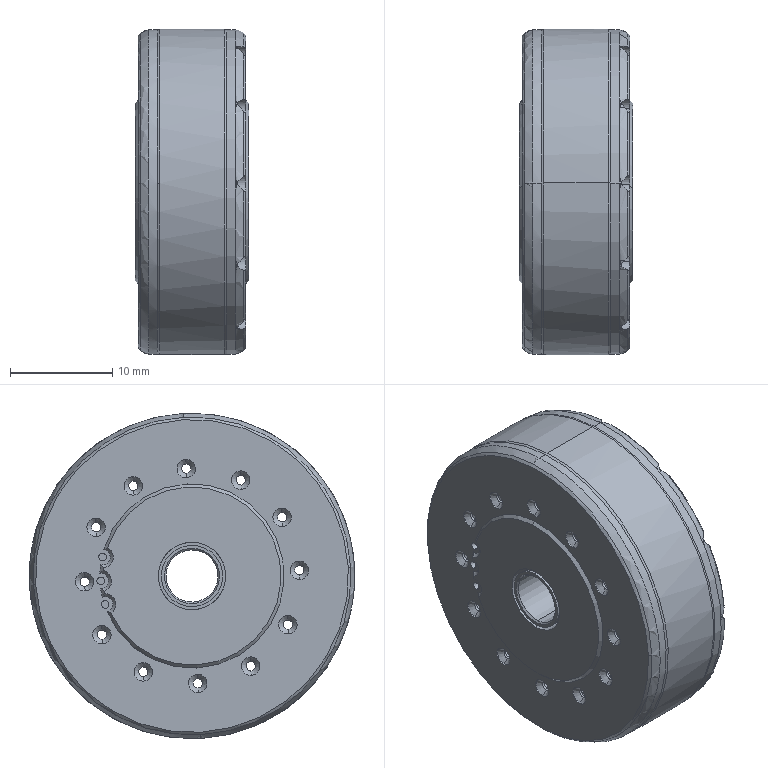Part | SolidWorks | features BaseBody 3, ICE 1, Scale 1 | 2 solids | 732 faces | box 11.1 x 31.8 x 31.8 mm | volume 3460 mm3 | cylinder 406 | plane 187 | cone 135 | spline 4 | commonest cylinder face diameters 0.9 x72 1.8 x72 24.899 x60 28.201 x32 24.6 x31 0.75 x30